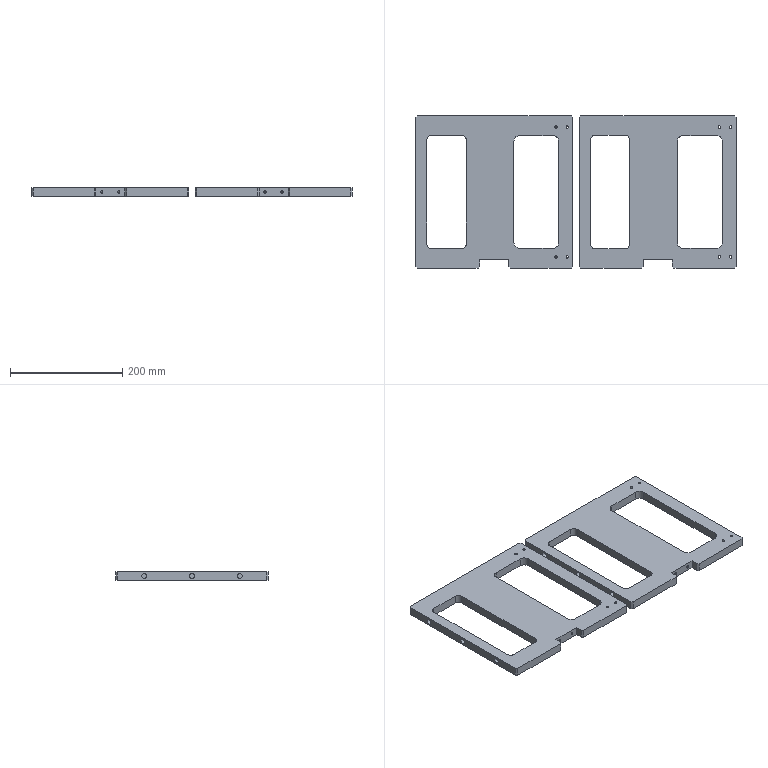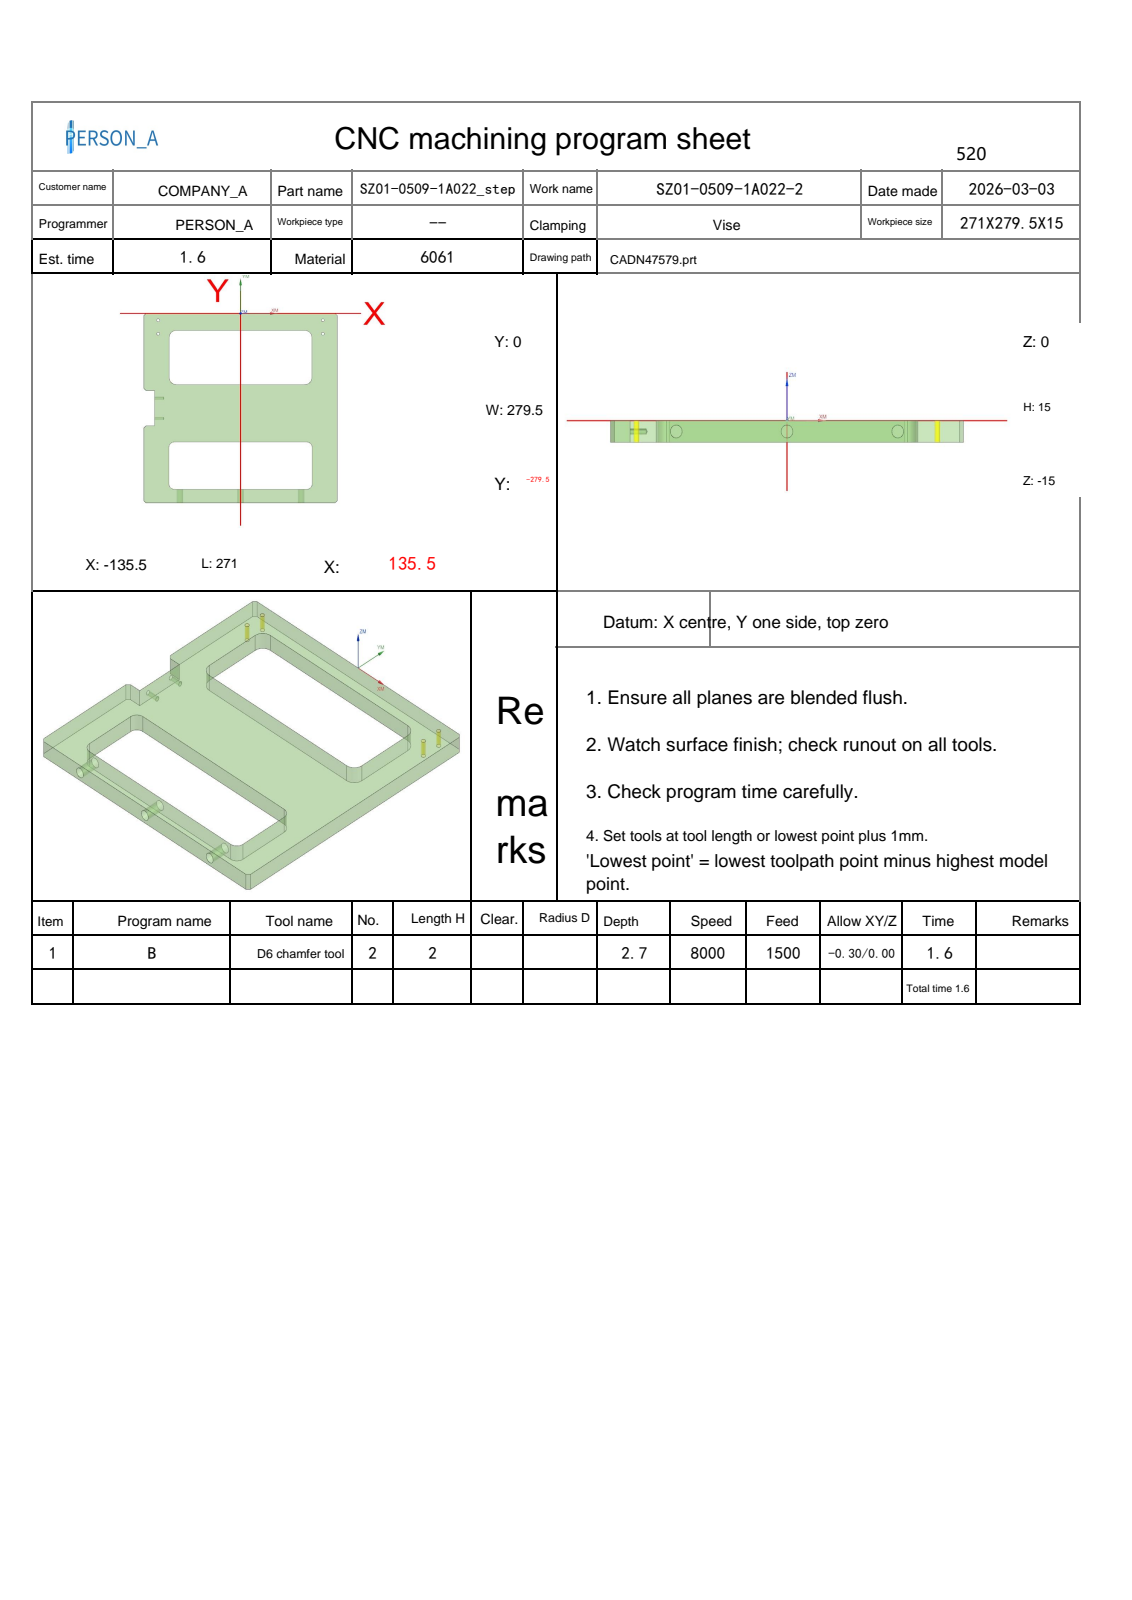NC program | NX | posted by the shop | part box 570 x 271 x 15 mm
Whole program:
%
O0001
(Machine time: 1.79 MIN)
(===Total Tool:1===)
(T2=D6 chamfer tool   D=6.   R=0.   D-  H02 Z=-2.7  )
G80 G90 G17 G49 G40
G91 G28 Z0
M01
N1 T02 M06
(D6 chamfer tool D=6. R=0. H=02 ce=-0.30 di=0.00)
G00 G90 G54 X-99.566 Y-253.332 M03 S7000
G43 H02 Z50.
M08
Z2.5
G01 X-99.543 Y-253.431 Z2.463 F1500.
X-99.367 Y-253.986 Z2.251
X-99.147 Y-254.524 Z2.04
X-98.886 Y-255.043 Z1.828
X-98.584 Y-255.54 Z1.616
X-98.243 Y-256.012 Z1.405
X-97.866 Y-256.454 Z1.193
X-97.454 Y-256.866 Z.981
X-97.012 Y-257.243 Z.77
X-96.54 Y-257.584 Z.558
X-96.043 Y-257.886 Z.346
X-95.524 Y-258.147 Z.135
X-94.986 Y-258.367 Z-.077
X-94.431 Y-258.543 Z-.289
X-93.865 Y-258.674 Z-.5
X-93.29 Y-258.76 Z-.712
X-92.709 Y-258.8 Z-.924
X-92.5 Z-1.
X92.5
G03 X99.8 Y-251.5 I0.0 J7.3
G01 Y-197.5
G03 X92.5 Y-190.2 I-7.3 J0.0
G01 X-92.5
G03 X-99.8 Y-197.5 I0.0 J-7.3
G01 Y-251.5
G03 X-92.5 Y-258.8 I7.3 J0.0
G01 X-92.
Z1.5
G00 Z50.
X-128.327 Y-280.2
Z2.5
G01 X-132.376 Z1.026
X-132.453 Z.998
X-132.66 Y-280.162 Z.921
X-132.855 Y-280.081 Z.845
X-133.028 Y-279.962 Z.768
X-135.962 Y-277.028 Z-.742
X-136.081 Y-276.855 Z-.819
X-136.162 Y-276.66 Z-.895
X-136.2 Y-276.453 Z-.972
Y-276.376 Z-1.
Y-168.874
G02 X-135.907 Y-168.167 I1. J0.0
G01 X-133.083 Y-165.343
G02 X-132.376 Y-165.05 I.707 J-.707
G01 X-121.2
Y-114.45
X-132.376
G02 X-133.083 Y-114.157 I0.0 J1.
G01 X-135.907 Y-111.333
G02 X-136.2 Y-110.626 I.707 J.707
G01 Y-3.124
G02 X-135.907 Y-2.417 I1. J0.0
G01 X-133.083 Y.407
G02 X-132.376 Y.7 I.707 J-.707
G01 X132.376
G02 X133.083 Y.407 I0.0 J-1.
G01 X135.907 Y-2.417
G02 X136.2 Y-3.124 I-.707 J-.707
G01 Y-276.376
G02 X135.907 Y-277.083 I-1. J0.0
G01 X133.083 Y-279.907
G02 X132.376 Y-280.2 I-.707 J.707
G01 X-132.376
G02 X-133.083 Y-279.907 I0.0 J1.
G01 X-135.907 Y-277.083
G02 X-136.2 Y-276.376 I.707 J.707
G01 Y-275.876
Z1.5
G00 Z50.
X-97.989 Y-99.756
Z2.5
G01 X-97.791 Y-100.084 Z2.361
X-97.422 Y-100.609 Z2.127
X-97.017 Y-101.108 Z1.893
X-96.578 Y-101.578 Z1.659
X-96.108 Y-102.017 Z1.425
X-95.609 Y-102.422 Z1.191
X-95.084 Y-102.791 Z.957
X-94.534 Y-103.124 Z.723
X-93.962 Y-103.417 Z.489
X-93.371 Y-103.671 Z.255
X-92.765 Y-103.883 Z.022
X-92.145 Y-104.052 Z-.212
X-91.515 Y-104.179 Z-.446
X-90.878 Y-104.262 Z-.68
X-90.236 Y-104.3 Z-.914
X-90. Z-1.
X90.
G03 X99.3 Y-95. I0.0 J9.3
G01 Y-35.
G03 X90. Y-25.7 I-9.3 J0.0
G01 X-90.
G03 X-99.3 Y-35. I0.0 J-9.3
G01 Y-95.
G03 X-90. Y-104.3 I9.3 J0.0
G01 X-89.5
Z1.5
G00 Z50.
G00 G90 X-115.5 Y-10. M03 S8000
Z50.
G98 G81 X-115.5 Y-10. Z-2.7 R3. F1000.
Y-30.
X115.5
Y-10.
G80
G00 Z50.
M05
M09
G91 G28 Z0.0
G91 G28 Y0.0
M30
%